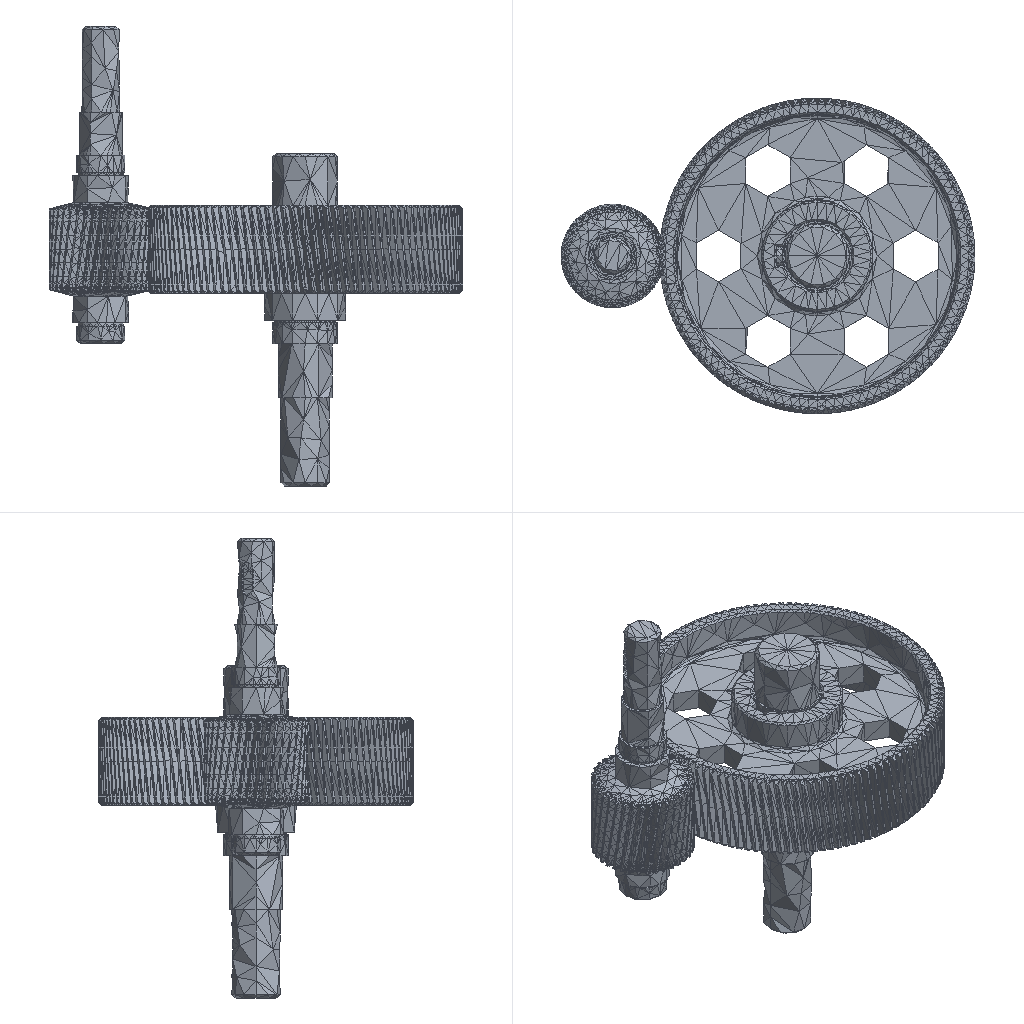Simulation study | ansys workbench
Set-up summary:
category,name,step,type,value,unit,region
solver,ansys_workbench
units,mm-N-s-tonne (MPa),,stated,"/units,MPA"
analysis,LS1,,transient
load_step,LS1,LS1,transient,time=1
load_step,LS2,LS2,transient,time=2
load_step,LS3,LS3,transient,time=3
load_step,LS4,LS4,transient,time=4
load_step,LS5,LS5,transient,time=5
mesh,nodes,,,43400
mesh,elements,,,25750
element_type,SOLID187,,,22515
element_type,CONTA174,,,2275
element_type,TARGE170,,,912
element_type,SOLID186,,,48
material,Structural Steel,,E,200000,tonne s^-2 mm^-1
material,Structural Steel,,nu,0.3
material,Structural Steel,,density,7.85e-09,tonne mm^-3
material,Structural Steel,,conductivity,60.5,tonne mm s^-3 C^-1
material,Structural Steel,,specific_heat,4.34e+08,mm^2 s^-2 C^-1
material,Structural Steel,,cte,1.2e-05,C^-1
material,Structural Steel,,permeability,10000
material,Structural Steel,,resistivity,0.00017,ohm mm
load,,LS1,moment,"720000 [dir=(0, 0, 1) n=3]",,all
bc,Fixed Supports,model,fixed,[dofs=ALL],,_FIXEDSU
contact,Contact Region,,bonded (always),element=CONTA174
contact,Contact Region 2,,bonded (always),element=CONTA174
contact,Contact Region 3,,bonded (always),element=CONTA174
contact,Contact Region 4,,bonded (always),element=CONTA174
contact,contact 5,,bonded (always),element=CONTA174
named_set,______,,node,5211
named_set,______,,node,4194
named_set,_FIXEDSU,,node,832
Ansys APDL input file, long lists of numbers shortened:
/batch
/config,noeldb,1     ! force off writing results to database
*get,_wallstrt,active,,time,wall
! ANSYS input file written by Workbench version 2022 R1
! File used for geometry attach:
/title,wbnew--__ (B5)
! ****** Begin Custom Load Command Snippet ******
/COM, ACT Extensions:
/COM,     LSDYNA, 2021.1
/COM,
! ****** End   Custom Load Command Snippet ******
*DIM,_wb_ProjectScratch_dir,string,248
_wb_ProjectScratch_dir(1) = ''
*DIM,_wb_SolverFiles_dir,string,248
_wb_SolverFiles_dir(1) = ''
*DIM,_wb_userfiles_dir,string,248
_wb_userfiles_dir(1) = ''
/com,--- Data in consistent NMM units. See Solving Units in the help system for more information.
/units,MPA
/nopr
/wb,file,start              !  signify a WB generated input file
/prep7
! Turn off shape checking because checks already performed inside WB mesher.
! See help system for more information.
SHPP,OFF,,NOWARN
/nolist
etcon,set             ! allow ANSYS to choose best KEYOP's for 180x elements, resets any applicable keyopt to MAPDL defaults
/com,*********** Nodes for the whole assembly ***********
nblock,3,,47738
(1i9,3e20.9e3)
        1    -1.142439996E+03    -8.863225486E+02     1.510414168E+03
! (43398 more lines like these left out)
-1
/com,*********** Nodes for all Remote Points ***********
nblock,3
(1i9,3e20.9e3)
    43400    -1.169440518E+03    -8.844112916E+02     1.421479178E+03
-1
/wb,elem,start            !  set before creation of elements
/com,*********** Elements for Body 1 "________|__-__2" ***********
et,1,187
eblock,19,solid,,11378
(19i9)
        1        1        1        1        0        0        0        0       10        0     2828     7985     8037     8695     8679    23877    24110    23882    23881
! (22755 more lines like these left out)
-1
/com,*********** Elements for Body 2 "___|__1" ***********
et,2,187
eblock,19,solid,,8358
(19i9)
        2        2        2        2        0        0        0        0       10        0    14206    27017    29013    29286    28871    32610    42362    32612    32609
! (16715 more lines like these left out)
-1
/com,*********** Elements for Body 3 "___|__1" ***********
et,3,187
eblock,19,solid,,2779
(19i9)
        3        3        3        3        0        0        0        0       10        0        1       84      100      757      684     1333     1469     1342     1337
! (5557 more lines like these left out)
-1
/com,*********** Elements for Body 4 "______|__-__1" ***********
et,4,186
keyo,4,2,1          ! set full integration on SOLID186
eblock,19,solid,,48
(19i9)
        4        4        4        4        0        0        0        0       20        0     2780     4788     4794     4789     4795     4815     4809     4814     4808
! (95 more lines like these left out)
-1
/wb,elem,end               !  done creating elements
/com,*********** Send User Defined Coordinate System(s) ***********
csys,0
toffst,273.15,  ! Temperature offset from absolute zero
/com,*********** Set Reference Temperature ***********
tref,22.
/wb,mat,start              !  starting to send materials
/com,*********** Send Materials ***********
Temperature = 'TEMP' ! Temperature
MP,DENS,1,7.85e-09,	! tonne mm^-3
MP,ALPX,1,1.2e-05,	! C^-1
MP,C,1,434000000,	! mm^2 s^-2 C^-1
MP,KXX,1,60.5,	! tonne mm s^-3 C^-1
MP,RSVX,1,0.00017,	! ohm mm
MP,EX,1,200000,	! tonne s^-2 mm^-1
MP,NUXY,1,0.3,
MP,MURX,1,10000,
Temperature = 'TEMP' ! Temperature
MP,DENS,2,7.85e-09,	! tonne mm^-3
MP,ALPX,2,1.2e-05,	! C^-1
MP,C,2,434000000,	! mm^2 s^-2 C^-1
MP,KXX,2,60.5,	! tonne mm s^-3 C^-1
MP,RSVX,2,0.00017,	! ohm mm
MP,EX,2,200000,	! tonne s^-2 mm^-1
MP,NUXY,2,0.3,
MP,MURX,2,10000,
Temperature = 'TEMP' ! Temperature
MP,DENS,3,7.85e-09,	! tonne mm^-3
MP,ALPX,3,1.2e-05,	! C^-1
MP,C,3,434000000,	! mm^2 s^-2 C^-1
MP,KXX,3,60.5,	! tonne mm s^-3 C^-1
MP,RSVX,3,0.00017,	! ohm mm
MP,EX,3,200000,	! tonne s^-2 mm^-1
MP,NUXY,3,0.3,
MP,MURX,3,10000,
Temperature = 'TEMP' ! Temperature
MP,DENS,4,7.85e-09,	! tonne mm^-3
MP,ALPX,4,1.2e-05,	! C^-1
MP,C,4,434000000,	! mm^2 s^-2 C^-1
MP,KXX,4,60.5,	! tonne mm s^-3 C^-1
MP,RSVX,4,0.00017,	! ohm mm
MP,EX,4,200000,	! tonne s^-2 mm^-1
MP,NUXY,4,0.3,
MP,MURX,4,10000,
/wb,mat,end                !  done sending materials
!************************* Model Summary ********************
!________|__-__2,	结构钢,	matid,	1
!___|__1,	结构钢,	matid,	2
!___|__1,	结构钢,	matid,	3
!______|__-__1,	结构钢,	matid,	4
!************************* End Model Summary ********************
! get the diagonal of the bounding box. Needed later for other things
*get,_xmin,node,,mnloc,x
*get,_ymin,node,,mnloc,y
*get,_zmin,node,,mnloc,z
*get,_xmax,node,,mxloc,x
*get,_ymax,node,,mxloc,y
*get,_zmax,node,,mxloc,z
_ASMDIAG=(_xmax-_xmin)*(_xmax-_xmin)+(_ymax-_ymin)*(_ymax-_ymin)+(_zmax-_zmin)*(_zmax-_zmin)
_ASMDIAG=SQRT(_ASMDIAG)
/wb,contact,start          !  starting to send contact
/com,*********** Create Contact "接触区域" ***********
/com,            Real Constant Set For Above Contact Is 6 & 5
*set,tid,6
*set,cid,5
r,tid
r,cid
et,tid,170
et,cid,174
eblock,10,,,368
(15i9)
    34695        6        6        6        0     6943     6956     7970     7970    19321    19378     7970    19324
! (367 more lines like these left out)
-1
eblock,10,,,368
(15i9)
    35063        5        5        5        0     6943     6956     7970     7970    19321    19378     7970    19324
! (367 more lines like these left out)
-1
eblock,10,,,70
(15i9)
    35431        5        6        5        0    27457    28630    27459    27459    34895    34904    27459    34894
! (69 more lines like these left out)
-1
eblock,10,,,70
(15i9)
    35501        6        5        6        0    27457    28630    27459    27459    34895    34904    27459    34894
! (69 more lines like these left out)
-1
keyo,cid,8,2               ! auto create asymmetric contact (from Program Controlled setting)
keyo,cid,10,0              ! adjust contact stiffness each NR iteration (from Program Controlled setting)
keyo,cid,12,5              ! bonded always
keyo,cid,18,1              ! small sliding turned on by application
keyo,cid,2,0               ! augmented Lagrange (from Program Controlled setting)
keyo,cid,4,0               ! on Gauss point (from Program Controlled setting)
keyo,cid,9,1               ! ignore initial gaps/penetration
keyo,cid,7,0               ! No Prediction
rmod,tid,3,10.      ! FKN
rmod,tid,5,0.       ! ICONT
rmod,tid,6,0.       ! PINB
rmod,tid,10,0.      ! CNOF
rmod,tid,12,0.      ! FKT
rmod,tid,36,35      ! WB DSID
rmod,cid,3,10.      ! FKN
rmod,cid,5,0.       ! ICONT
rmod,cid,6,0.       ! PINB
rmod,cid,10,0.      ! CNOF
rmod,cid,12,0.      ! FKT
rmod,cid,36,35      ! WB DSID
/com,*********** Create Contact "接触区域 2" ***********
/com,            Real Constant Set For Above Contact Is 8 & 7
*set,tid,8
*set,cid,7
r,tid
r,cid
et,tid,170
et,cid,174
eblock,10,,,134
(15i9)
    35571        8        8        8        0    26777    28864    28922    28922    31185    41775    28922    31186
! (133 more lines like these left out)
-1
eblock,10,,,134
(15i9)
    35705        7        7        7        0    26777    28864    28922    28922    31185    41775    28922    31186
! (133 more lines like these left out)
-1
eblock,10,,,130
(15i9)
    35839        7        8        7        0       53      280      436      436     1073     2676      436     1074
! (129 more lines like these left out)
-1
eblock,10,,,130
(15i9)
    35969        8        7        8        0       53      280      436      436     1073     2676      436     1074
! (129 more lines like these left out)
-1
keyo,cid,8,2               ! auto create asymmetric contact (from Program Controlled setting)
keyo,cid,10,0              ! adjust contact stiffness each NR iteration (from Program Controlled setting)
keyo,cid,12,5              ! bonded always
keyo,cid,18,1              ! small sliding turned on by application
keyo,cid,2,0               ! augmented Lagrange (from Program Controlled setting)
keyo,cid,4,0               ! on Gauss point (from Program Controlled setting)
keyo,cid,9,1               ! ignore initial gaps/penetration
keyo,cid,7,0               ! No Prediction
rmod,tid,3,10.      ! FKN
rmod,tid,5,0.       ! ICONT
rmod,tid,6,0.       ! PINB
rmod,tid,10,0.      ! CNOF
rmod,tid,12,0.      ! FKT
rmod,tid,36,38      ! WB DSID
rmod,cid,3,10.      ! FKN
rmod,cid,5,0.       ! ICONT
rmod,cid,6,0.       ! PINB
rmod,cid,10,0.      ! CNOF
rmod,cid,12,0.      ! FKT
rmod,cid,36,38      ! WB DSID
/com,*********** Create Contact "接触区域 3" ***********
/com,            Real Constant Set For Above Contact Is 10 & 9
*set,tid,10
*set,cid,9
r,tid
r,cid
et,tid,170
et,cid,174
eblock,10,,,38
(15i9)
    36099       10       10       10        0    26939    28634    28947    28947    32120    40618    28947    32122
! (37 more lines like these left out)
-1
eblock,10,,,38
(15i9)
    36137        9        9        9        0    26939    28634    28947    28947    32120    40618    28947    32122
! (37 more lines like these left out)
-1
eblock,10,,,64
(15i9)
    36175        9       10        9        0     4857     4852     4851     4849     5078     5075     5071     5072
! (63 more lines like these left out)
-1
eblock,10,,,64
(15i9)
    36239       10        9       10        0     4857     4852     4851     4849     5078     5075     5071     5072
! (63 more lines like these left out)
-1
keyo,cid,8,2               ! auto create asymmetric contact (from Program Controlled setting)
keyo,cid,10,0              ! adjust contact stiffness each NR iteration (from Program Controlled setting)
keyo,cid,12,5              ! bonded always
keyo,cid,18,1              ! small sliding turned on by application
keyo,cid,2,0               ! augmented Lagrange (from Program Controlled setting)
keyo,cid,4,0               ! on Gauss point (from Program Controlled setting)
keyo,cid,9,1               ! ignore initial gaps/penetration
keyo,cid,7,0               ! No Prediction
rmod,tid,3,10.      ! FKN
rmod,tid,5,0.       ! ICONT
rmod,tid,6,0.       ! PINB
rmod,tid,10,0.      ! CNOF
rmod,tid,12,0.      ! FKT
rmod,tid,36,41      ! WB DSID
rmod,cid,3,10.      ! FKN
rmod,cid,5,0.       ! ICONT
rmod,cid,6,0.       ! PINB
rmod,cid,10,0.      ! CNOF
rmod,cid,12,0.      ! FKT
rmod,cid,36,41      ! WB DSID
/com,*********** Create Contact "接触区域 4" ***********
/com,            Real Constant Set For Above Contact Is 12 & 11
*set,tid,12
*set,cid,11
r,tid
r,cid
et,tid,170
et,cid,174
eblock,10,,,44
(15i9)
    36303       12       12       12        0       35       32       33       33      917      916       33      927
! (43 more lines like these left out)
-1
eblock,10,,,44
(15i9)
    36347       11       11       11        0       35       32       33       33      917      916       33      927
! (43 more lines like these left out)
-1
eblock,10,,,64
(15i9)
    36391       11       12       11        0     4857     4852     4851     4849     5078     5075     5071     5072
! (63 more lines like these left out)
-1
eblock,10,,,64
(15i9)
    36455       12       11       12        0     4857     4852     4851     4849     5078     5075     5071     5072
! (63 more lines like these left out)
-1
keyo,cid,8,2               ! auto create asymmetric contact (from Program Controlled setting)
keyo,cid,10,0              ! adjust contact stiffness each NR iteration (from Program Controlled setting)
keyo,cid,12,5              ! bonded always
keyo,cid,18,1              ! small sliding turned on by application
keyo,cid,2,0               ! augmented Lagrange (from Program Controlled setting)
keyo,cid,4,0               ! on Gauss point (from Program Controlled setting)
keyo,cid,9,1               ! ignore initial gaps/penetration
keyo,cid,7,0               ! No Prediction
rmod,tid,3,10.      ! FKN
rmod,tid,5,0.       ! ICONT
rmod,tid,6,0.       ! PINB
rmod,tid,10,0.      ! CNOF
rmod,tid,12,0.      ! FKT
rmod,tid,36,44      ! WB DSID
rmod,cid,3,10.      ! FKN
rmod,cid,5,0.       ! ICONT
rmod,cid,6,0.       ! PINB
rmod,cid,10,0.      ! CNOF
rmod,cid,12,0.      ! FKT
rmod,cid,36,44      ! WB DSID
nsel,all
esel,all
/wb,contact,end            !  done creating contacts
/com,*********** Send Named Selection as Node Component ***********
CMBLOCK,______  ,NODE,     5211
(8i10)
      5183      5184      5189      5191      5192      5193      5198      5201
! (651 more lines like these left out)
/com,*********** Send Named Selection as Node Component ***********
CMBLOCK,______  ,NODE,     4194
(8i10)
     26944     26946     27058     27059     27060     27061     27062     27063
! (524 more lines like these left out)
/golist
/wb,load,start             !  starting to send loads
/com,*********** Fixed Supports ***********
CMBLOCK,_FIXEDSU,NODE,      832
(8i10)
         9        10        11        12        13        14        15        16
! (103 more lines like these left out)
cmsel,s,_FIXEDSU
d,all,all
nsel,all
/com,*********** Create Remote Point "内部远程点" ***********
! -------- Remote Point Used by "力矩" --------
*set,tid,14
*set,cid,13
et,cid,174
et,tid,170
keyo,tid,2,1               ! Don't fix the pilot node
keyo,tid,4,0               ! Activate all DOF's due to large deformation
keyo,cid,12,5              ! Bonded Contact
keyo,cid,4,1               ! Deformable RBE3 style load
keyo,cid,2,2               ! MPC style contact
eblock,10,,,1363
(15i9)
    36519       13       13       13        0    28120    28130    28129    28129    38352    38395    28129    38351
! (1362 more lines like these left out)
-1
*set,_npilot,43400
_npilot67=_npilot
type,tid
mat ,cid
real,cid
tshape,pilo
en,37882,_npilot
tshape
/com,*********** Construct Moment Using Remote Attachment ***********
/gst,on,on
fini
*get,_numnode,node,0,count
*get,_numelem,elem,0,count
*get, _MAXELEMNUM, elem, 0, NUM, MAX
*get, _MAXNODENUM, node, 0, NUM, MAX
*get, _MAXELEMTYPE, etyp, 0, NUM, MAX
*get, _MAXREALCONST, real, 0, NUM, MAX
/go
/wb,load,end               !  done creating loads
/com,--- Number of total nodes = %_numnode%
/com,--- Number of contact elements = 3187
/com,--- Number of spring elements = 0
/com,--- Number of bearing elements = 0
/com,--- Number of solid elements = 22563
/com,--- Number of condensed parts = 0
/com,--- Number of total elements = %_numelem%
*get,_wallbsol,active,,time,wall
/com,****************************************************************************
/com,*************************    SOLUTION       ********************************
/com,****************************************************************************
/solu
antype,4                   ! transient analysis
nlgeom,on                  ! Turn on Large Deformation Effects
kbc,1                      ! stepped BC's
_thickRatio=0.5     ! Ratio of thick parts in the model
eqsl,sparse,,,,,1
cntr,print,1               ! print out contact info and also make no initial contact an error
dmpoption,emat,no             ! Don't combine emat file for DANSYS
dmpoption,esav,no             ! Don't combine esav file for DANSYS
trnopt,full,,,,,hht        ! HHT time integration method
tintp, mosp			! Choose transient integration settings for moderate speed application
nldiag,cont,iter           ! print out contact info each equilibrium iteration
rescontrol,define,last,last,,dele	   ! Program Controlled
/com,****************************************************
/com,******************* SOLVE FOR LS 1 OF 5 ****************
nsel,s,node,,43400
f,all,mx,0.
f,all,my,0.
f,all,mz,720000.
nsel,all
/nopr
/gopr
autots,on                   ! User turned on automatic time stepping
deltim,1,1,1,OFF
time,1.
timint,on                  ! Turn on time integration effects
outres,erase
outres,all,none
outres,nsol,all,
outres,rsol,all
outres,eangl,all
outres,etmp,all
outres,veng,all
outres,strs,all,
outres,epel,all,
outres,eppl,all,
outres,cont,all,
outres,v,all,
outres,a,all,
! *********** WB SOLVE COMMAND ***********
! check interactive state
*get,ANSINTER_,active,,int
*if,ANSINTER_,ne,0,then
/eof
*endif
solve
/com *************** Write FE CONNECTORS *********
CEWRITE,file,ce,,INTE
/com,****************************************************
/com,*************** FINISHED SOLVE FOR LS 1 *************
/com,****************************************************
/com,******************* SOLVE FOR LS 2 OF 5 ****************
/nopr
/gopr
autots,on                   ! User turned on automatic time stepping
deltim,1,1,1,OFF
time,2.
timint,on                  ! Turn on time integration effects
outres,erase
outres,all,none
outres,nsol,all,
outres,rsol,all
outres,eangl,all
outres,etmp,all
outres,veng,all
outres,strs,all,
outres,epel,all,
outres,eppl,all,
outres,cont,all,
outres,v,all,
outres,a,all,
solve
/com,****************************************************
/com,*************** FINISHED SOLVE FOR LS 2 *************
/com,****************************************************
/com,******************* SOLVE FOR LS 3 OF 5 ****************
/nopr
/gopr
autots,on                   ! User turned on automatic time stepping
deltim,1,1,1,OFF
time,3.
timint,on                  ! Turn on time integration effects
outres,erase
outres,all,none
outres,nsol,all,
outres,rsol,all
outres,eangl,all
outres,etmp,all
outres,veng,all
outres,strs,all,
outres,epel,all,
outres,eppl,all,
outres,cont,all,
outres,v,all,
outres,a,all,
solve
/com,****************************************************
/com,*************** FINISHED SOLVE FOR LS 3 *************
/com,****************************************************
/com,******************* SOLVE FOR LS 4 OF 5 ****************
/nopr
/gopr
autots,on                   ! User turned on automatic time stepping
deltim,1,1,1,OFF
time,4.
timint,on                  ! Turn on time integration effects
outres,erase
outres,all,none
outres,nsol,all,
outres,rsol,all
outres,eangl,all
outres,etmp,all
outres,veng,all
outres,strs,all,
outres,epel,all,
outres,eppl,all,
outres,cont,all,
outres,v,all,
outres,a,all,
solve
/com,****************************************************
/com,*************** FINISHED SOLVE FOR LS 4 *************
/com,****************************************************
/com,******************* SOLVE FOR LS 5 OF 5 ****************
/nopr
/gopr
autots,on                   ! User turned on automatic time stepping
deltim,1,1,1,OFF
time,5.
timint,on                  ! Turn on time integration effects
outres,erase
outres,all,none
outres,nsol,all,
outres,rsol,all
outres,eangl,all
outres,etmp,all
outres,veng,all
outres,strs,all,
outres,epel,all,
outres,eppl,all,
outres,cont,all,
outres,v,all,
outres,a,all,
solve
/com,****************************************************
/com,*************** FINISHED SOLVE FOR LS 5 *************
*get,_wallasol,active,,time,wall
/nopr
*get,_numnode,node,0,count
*get,_numelem,elem,0,count
*get, _MAXELEMNUM, elem, 0, NUM, MAX
*get, _MAXNODENUM, node, 0, NUM, MAX,,,INTERNAL
*get, _MAXELEMTYPE, etyp, 0, NUM, MAX
*get, _MAXREALCONST, real, 0, NUM, MAX
/gopr
/post1
xmlo,ENCODING,ISO-8859-1
xmlo,parm
/xml,parm,xml
fini
/gopr
*get,_walldone,active,,time,wall
_preptime=(_wallbsol-_wallstrt)*3600
_solvtime=(_wallasol-_wallbsol)*3600
_posttime=(_walldone-_wallasol)*3600
_totaltim=(_walldone-_wallstrt)*3600
*get,_dlbratio,active,0,solu,dlbr
*get,_combtime,active,0,solu,comb
*get,_ssmode,active,0,solu,ssmm
*get,_ndofs,active,0,solu,ndof
*get,_sol_end_time,active,0,set,time
*if,_sol_end_time,eq,5.,then
/fclean				!clean distributed files
*endif
/com,--- Total number of nodes = %_numnode%
/com,--- Total number of elements = %_numelem%
/com,--- Element load balance ratio = %_dlbratio%
/com,--- Time to combine distributed files = %_combtime%
/com,--- Sparse memory mode = %_ssmode%
/com,--- Number of DOF = %_ndofs%
/wb,file,end               ! done with WB generated input
Results summary:
result,analyses[0].index,,,1
result,analyses[0].system,,,SYS
result,analyses[0].deck,,,deck.dat
result,analyses[0].solve_status,,,completed
result,analyses[0].analysis_type,,,static
result,analyses[0].physics,,,mechanical
result,analyses[0].unit_system,,,"NMM: mm, ton, N, s, mV, mA, degC"
result,analyses[0].n_sets,,,5
result,analyses[0].load_steps[0].set,set=1,,1
result,analyses[0].load_steps[0].time_or_freq,set=1,,1
result,analyses[0].load_steps[0].max_displacement_magnitude,set=1,,0.007305
result,analyses[0].load_steps[0].max_von_mises_nodal,set=1,,24.097
result,analyses[0].load_steps[0].reaction_force_sum_xyz[1],set=1,,-9.24116e-06
result,analyses[0].load_steps[0].reaction_force_sum_xyz[2],set=1,,4.27889e-05
result,analyses[0].load_steps[0].reaction_force_sum_xyz[3],set=1,,-1.34164e-05
result,analyses[0].load_steps[1].set,set=2,,2
result,analyses[0].load_steps[1].time_or_freq,set=2,,2
result,analyses[0].load_steps[1].max_displacement_magnitude,set=2,,0.007305
result,analyses[0].load_steps[1].max_von_mises_nodal,set=2,,24.097
result,analyses[0].load_steps[1].reaction_force_sum_xyz[1],set=2,,3.53161e-05
result,analyses[0].load_steps[1].reaction_force_sum_xyz[2],set=2,,-0.0001235
result,analyses[0].load_steps[1].reaction_force_sum_xyz[3],set=2,,-9.52615e-06
result,analyses[0].load_steps[2].set,set=3,,3
result,analyses[0].load_steps[2].time_or_freq,set=3,,3
result,analyses[0].load_steps[2].max_displacement_magnitude,set=3,,0.007305
result,analyses[0].load_steps[2].max_von_mises_nodal,set=3,,24.097
result,analyses[0].load_steps[2].reaction_force_sum_xyz[1],set=3,,-4.83163e-05
result,analyses[0].load_steps[2].reaction_force_sum_xyz[2],set=3,,0.0001783
result,analyses[0].load_steps[2].reaction_force_sum_xyz[3],set=3,,-1.8251e-05
result,analyses[0].load_steps[3].set,set=4,,4
result,analyses[0].load_steps[3].time_or_freq,set=4,,4
result,analyses[0].load_steps[3].max_displacement_magnitude,set=4,,0.007305
result,analyses[0].load_steps[3].max_von_mises_nodal,set=4,,24.097
result,analyses[0].load_steps[3].reaction_force_sum_xyz[1],set=4,,4.79161e-05
result,analyses[0].load_steps[3].reaction_force_sum_xyz[2],set=4,,-0.0002093
result,analyses[0].load_steps[3].reaction_force_sum_xyz[3],set=4,,-7.72812e-06
result,analyses[0].load_steps[4].set,set=5,,5
result,analyses[0].load_steps[4].time_or_freq,set=5,,5
result,analyses[0].load_steps[4].max_displacement_magnitude,set=5,,0.007305
result,analyses[0].load_steps[4].max_von_mises_nodal,set=5,,24.097
result,analyses[0].load_steps[4].reaction_force_sum_xyz[1],set=5,,-4.62078e-05
result,analyses[0].load_steps[4].reaction_force_sum_xyz[2],set=5,,0.0002241
result,analyses[0].load_steps[4].reaction_force_sum_xyz[3],set=5,,-1.787e-05